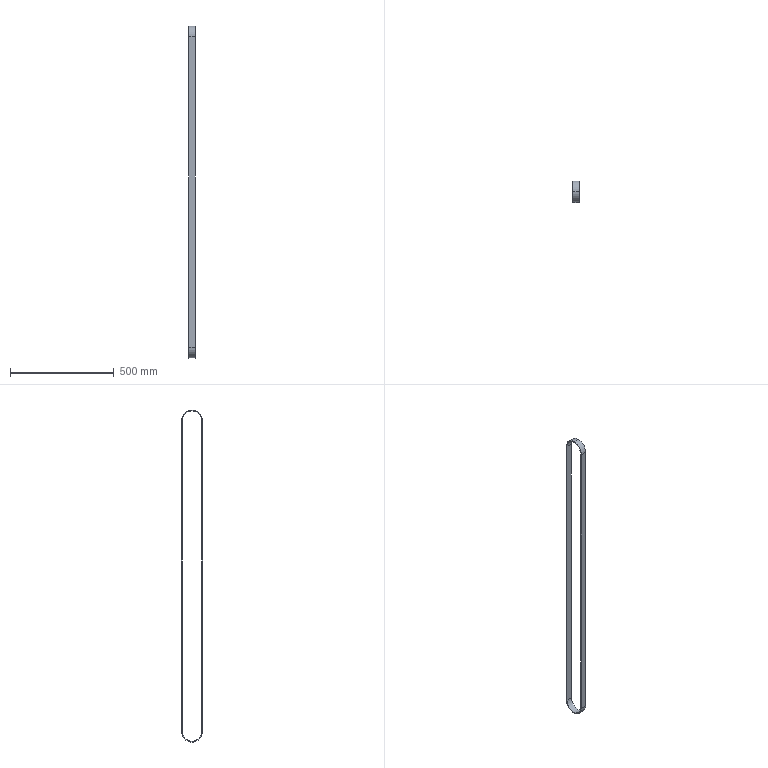Part | SolidWorks | features ExtruThin 1 | 1 solid | 12 faces | box 30 x 102.5 x 1599 mm | volume 445594 mm3 | cylinder 6 | plane 6 | commonest cylinder face diameters 93.5 x3 102.5 x3
STEP:
#1=CARTESIAN_POINT('',(15.,46.75,1496.41));
#2=VERTEX_POINT('',#1);
#3=CARTESIAN_POINT('',(15.,0.,1543.16));
#4=VERTEX_POINT('',#3);
#5=CARTESIAN_POINT('',(15.,0.,1496.41));
#6=DIRECTION('',(1.,0.,0.));
#7=DIRECTION('',(0.,0.,-1.));
#8=AXIS2_PLACEMENT_3D('',#5,#6,#7);
#9=CIRCLE('',#8,46.75);
#10=EDGE_CURVE('',#2,#4,#9,.T.);
#11=ORIENTED_EDGE('',*,*,#10,.T.);
#12=CARTESIAN_POINT('',(-15.,0.,1543.16));
#13=VERTEX_POINT('',#12);
#14=CARTESIAN_POINT('',(15.,0.,1543.16));
#15=DIRECTION('',(-1.,0.,0.));
#16=VECTOR('',#15,1000.);
#17=LINE('',#14,#16);
#18=EDGE_CURVE('',#4,#13,#17,.T.);
#19=ORIENTED_EDGE('',*,*,#18,.T.);
#20=CARTESIAN_POINT('',(-15.,46.75,1496.41));
#21=VERTEX_POINT('',#20);
#22=CARTESIAN_POINT('',(-15.,0.,1496.41));
#23=DIRECTION('',(1.,0.,0.));
#24=DIRECTION('',(0.,0.,-1.));
#25=AXIS2_PLACEMENT_3D('',#22,#23,#24);
#26=CIRCLE('',#25,46.75);
#27=EDGE_CURVE('',#21,#13,#26,.T.);
#28=ORIENTED_EDGE('',*,*,#27,.F.);
#29=CARTESIAN_POINT('',(15.,46.75,1496.41));
#30=DIRECTION('',(-1.,0.,0.));
#31=VECTOR('',#30,1000.);
#32=LINE('',#29,#31);
#33=EDGE_CURVE('',#2,#21,#32,.T.);
#34=ORIENTED_EDGE('',*,*,#33,.F.);
#35=EDGE_LOOP('',(#11,#19,#28,#34));
#36=FACE_OUTER_BOUND('',#35,.T.);
#37=CARTESIAN_POINT('',(15.,0.,1496.41));
#38=DIRECTION('',(-1.,0.,0.));
#39=DIRECTION('',(0.,0.,1.));
#40=AXIS2_PLACEMENT_3D('',#37,#38,#39);
#41=CYLINDRICAL_SURFACE('',#40,46.75);
#42=ADVANCED_FACE('',(#36),#41,.F.);
#43=CARTESIAN_POINT('',(15.,0.,1547.66));
#44=VERTEX_POINT('',#43);
#45=CARTESIAN_POINT('',(15.,-51.25,1496.41));
#46=VERTEX_POINT('',#45);
#47=CARTESIAN_POINT('',(15.,0.,1496.41));
#48=DIRECTION('',(1.,0.,0.));
#49=DIRECTION('',(0.,0.,-1.));
#50=AXIS2_PLACEMENT_3D('',#47,#48,#49);
#51=CIRCLE('',#50,51.25);
#52=EDGE_CURVE('',#44,#46,#51,.T.);
#53=ORIENTED_EDGE('',*,*,#52,.F.);
#54=CARTESIAN_POINT('',(-15.,0.,1547.66));
#55=VERTEX_POINT('',#54);
#56=CARTESIAN_POINT('',(15.,0.,1547.66));
#57=DIRECTION('',(-1.,0.,0.));
#58=VECTOR('',#57,1000.);
#59=LINE('',#56,#58);
#60=EDGE_CURVE('',#44,#55,#59,.T.);
#61=ORIENTED_EDGE('',*,*,#60,.T.);
#62=CARTESIAN_POINT('',(-15.,-51.25,1496.41));
#63=VERTEX_POINT('',#62);
#64=CARTESIAN_POINT('',(-15.,0.,1496.41));
#65=DIRECTION('',(1.,0.,0.));
#66=DIRECTION('',(0.,0.,-1.));
#67=AXIS2_PLACEMENT_3D('',#64,#65,#66);
#68=CIRCLE('',#67,51.25);
#69=EDGE_CURVE('',#55,#63,#68,.T.);
#70=ORIENTED_EDGE('',*,*,#69,.T.);
#71=CARTESIAN_POINT('',(15.,-51.25,1496.41));
#72=DIRECTION('',(-1.,0.,0.));
#73=VECTOR('',#72,1000.);
#74=LINE('',#71,#73);
#75=EDGE_CURVE('',#46,#63,#74,.T.);
#76=ORIENTED_EDGE('',*,*,#75,.F.);
#77=EDGE_LOOP('',(#53,#61,#70,#76));
#78=FACE_OUTER_BOUND('',#77,.T.);
#79=CARTESIAN_POINT('',(15.,0.,1496.41));
#80=DIRECTION('',(-1.,0.,0.));
#81=DIRECTION('',(0.,0.,1.));
#82=AXIS2_PLACEMENT_3D('',#79,#80,#81);
#83=CYLINDRICAL_SURFACE('',#82,51.25);
#84=ADVANCED_FACE('',(#78),#83,.T.);
#85=CARTESIAN_POINT('',(15.,51.25,1496.41));
#86=VERTEX_POINT('',#85);
#87=CARTESIAN_POINT('',(15.,0.,1496.41));
#88=DIRECTION('',(1.,0.,0.));
#89=DIRECTION('',(0.,0.,-1.));
#90=AXIS2_PLACEMENT_3D('',#87,#88,#89);
#91=CIRCLE('',#90,51.25);
#92=EDGE_CURVE('',#86,#44,#91,.T.);
#93=ORIENTED_EDGE('',*,*,#92,.T.);
#94=ORIENTED_EDGE('',*,*,#52,.T.);
#95=CARTESIAN_POINT('',(15.,-51.25,0.));
#96=VERTEX_POINT('',#95);
#97=CARTESIAN_POINT('',(15.,-51.25,1496.41));
#98=DIRECTION('',(0.,0.,-1.));
#99=VECTOR('',#98,1000.);
#100=LINE('',#97,#99);
#101=EDGE_CURVE('',#46,#96,#100,.T.);
#102=ORIENTED_EDGE('',*,*,#101,.T.);
#103=CARTESIAN_POINT('',(15.,51.25,0.));
#104=VERTEX_POINT('',#103);
#105=CARTESIAN_POINT('',(15.,0.,0.));
#106=DIRECTION('',(1.,0.,0.));
#107=DIRECTION('',(0.,0.,-1.));
#108=AXIS2_PLACEMENT_3D('',#105,#106,#107);
#109=CIRCLE('',#108,51.25);
#110=EDGE_CURVE('',#96,#104,#109,.T.);
#111=ORIENTED_EDGE('',*,*,#110,.T.);
#112=CARTESIAN_POINT('',(15.,51.25,0.));
#113=DIRECTION('',(0.,0.,1.));
#114=VECTOR('',#113,1000.);
#115=LINE('',#112,#114);
#116=EDGE_CURVE('',#104,#86,#115,.T.);
#117=ORIENTED_EDGE('',*,*,#116,.T.);
#118=EDGE_LOOP('',(#93,#94,#102,#111,#117));
#119=FACE_OUTER_BOUND('',#118,.T.);
#120=CARTESIAN_POINT('',(15.,-46.75,1496.41));
#121=VERTEX_POINT('',#120);
#122=CARTESIAN_POINT('',(15.,-46.75,0.));
#123=VERTEX_POINT('',#122);
#124=CARTESIAN_POINT('',(15.,-46.75,1496.41));
#125=DIRECTION('',(0.,0.,-1.));
#126=VECTOR('',#125,1000.);
#127=LINE('',#124,#126);
#128=EDGE_CURVE('',#121,#123,#127,.T.);
#129=ORIENTED_EDGE('',*,*,#128,.F.);
#130=CARTESIAN_POINT('',(15.,0.,1496.41));
#131=DIRECTION('',(1.,0.,0.));
#132=DIRECTION('',(0.,0.,-1.));
#133=AXIS2_PLACEMENT_3D('',#130,#131,#132);
#134=CIRCLE('',#133,46.75);
#135=EDGE_CURVE('',#4,#121,#134,.T.);
#136=ORIENTED_EDGE('',*,*,#135,.F.);
#137=ORIENTED_EDGE('',*,*,#10,.F.);
#138=CARTESIAN_POINT('',(15.,46.75,0.));
#139=VERTEX_POINT('',#138);
#140=CARTESIAN_POINT('',(15.,46.75,0.));
#141=DIRECTION('',(0.,0.,1.));
#142=VECTOR('',#141,1000.);
#143=LINE('',#140,#142);
#144=EDGE_CURVE('',#139,#2,#143,.T.);
#145=ORIENTED_EDGE('',*,*,#144,.F.);
#146=CARTESIAN_POINT('',(15.,0.,0.));
#147=DIRECTION('',(1.,0.,0.));
#148=DIRECTION('',(0.,0.,-1.));
#149=AXIS2_PLACEMENT_3D('',#146,#147,#148);
#150=CIRCLE('',#149,46.75);
#151=EDGE_CURVE('',#123,#139,#150,.T.);
#152=ORIENTED_EDGE('',*,*,#151,.F.);
#153=EDGE_LOOP('',(#129,#136,#137,#145,#152));
#154=FACE_BOUND('',#153,.T.);
#155=CARTESIAN_POINT('',(15.,0.,1496.41));
#156=DIRECTION('',(1.,0.,0.));
#157=DIRECTION('',(0.,0.,-1.));
#158=AXIS2_PLACEMENT_3D('',#155,#156,#157);
#159=PLANE('',#158);
#160=ADVANCED_FACE('',(#119,#154),#159,.T.);
#161=CARTESIAN_POINT('',(-15.,51.25,1496.41));
#162=VERTEX_POINT('',#161);
#163=CARTESIAN_POINT('',(-15.,0.,1496.41));
#164=DIRECTION('',(1.,0.,0.));
#165=DIRECTION('',(0.,0.,-1.));
#166=AXIS2_PLACEMENT_3D('',#163,#164,#165);
#167=CIRCLE('',#166,51.25);
#168=EDGE_CURVE('',#162,#55,#167,.T.);
#169=ORIENTED_EDGE('',*,*,#168,.F.);
#170=CARTESIAN_POINT('',(-15.,51.25,0.));
#171=VERTEX_POINT('',#170);
#172=CARTESIAN_POINT('',(-15.,51.25,0.));
#173=DIRECTION('',(0.,0.,1.));
#174=VECTOR('',#173,1000.);
#175=LINE('',#172,#174);
#176=EDGE_CURVE('',#171,#162,#175,.T.);
#177=ORIENTED_EDGE('',*,*,#176,.F.);
#178=CARTESIAN_POINT('',(-15.,-51.25,0.));
#179=VERTEX_POINT('',#178);
#180=CARTESIAN_POINT('',(-15.,0.,0.));
#181=DIRECTION('',(1.,0.,0.));
#182=DIRECTION('',(0.,0.,-1.));
#183=AXIS2_PLACEMENT_3D('',#180,#181,#182);
#184=CIRCLE('',#183,51.25);
#185=EDGE_CURVE('',#179,#171,#184,.T.);
#186=ORIENTED_EDGE('',*,*,#185,.F.);
#187=CARTESIAN_POINT('',(-15.,-51.25,1496.41));
#188=DIRECTION('',(0.,0.,-1.));
#189=VECTOR('',#188,1000.);
#190=LINE('',#187,#189);
#191=EDGE_CURVE('',#63,#179,#190,.T.);
#192=ORIENTED_EDGE('',*,*,#191,.F.);
#193=ORIENTED_EDGE('',*,*,#69,.F.);
#194=EDGE_LOOP('',(#169,#177,#186,#192,#193));
#195=FACE_OUTER_BOUND('',#194,.T.);
#196=ORIENTED_EDGE('',*,*,#27,.T.);
#197=CARTESIAN_POINT('',(-15.,-46.75,1496.41));
#198=VERTEX_POINT('',#197);
#199=CARTESIAN_POINT('',(-15.,0.,1496.41));
#200=DIRECTION('',(1.,0.,0.));
#201=DIRECTION('',(0.,0.,-1.));
#202=AXIS2_PLACEMENT_3D('',#199,#200,#201);
#203=CIRCLE('',#202,46.75);
#204=EDGE_CURVE('',#13,#198,#203,.T.);
#205=ORIENTED_EDGE('',*,*,#204,.T.);
#206=CARTESIAN_POINT('',(-15.,-46.75,0.));
#207=VERTEX_POINT('',#206);
#208=CARTESIAN_POINT('',(-15.,-46.75,1496.41));
#209=DIRECTION('',(0.,0.,-1.));
#210=VECTOR('',#209,1000.);
#211=LINE('',#208,#210);
#212=EDGE_CURVE('',#198,#207,#211,.T.);
#213=ORIENTED_EDGE('',*,*,#212,.T.);
#214=CARTESIAN_POINT('',(-15.,46.75,0.));
#215=VERTEX_POINT('',#214);
#216=CARTESIAN_POINT('',(-15.,0.,0.));
#217=DIRECTION('',(1.,0.,0.));
#218=DIRECTION('',(0.,0.,-1.));
#219=AXIS2_PLACEMENT_3D('',#216,#217,#218);
#220=CIRCLE('',#219,46.75);
#221=EDGE_CURVE('',#207,#215,#220,.T.);
#222=ORIENTED_EDGE('',*,*,#221,.T.);
#223=CARTESIAN_POINT('',(-15.,46.75,0.));
#224=DIRECTION('',(0.,0.,1.));
#225=VECTOR('',#224,1000.);
#226=LINE('',#223,#225);
#227=EDGE_CURVE('',#215,#21,#226,.T.);
#228=ORIENTED_EDGE('',*,*,#227,.T.);
#229=EDGE_LOOP('',(#196,#205,#213,#222,#228));
#230=FACE_BOUND('',#229,.T.);
#231=CARTESIAN_POINT('',(-15.,0.,1496.41));
#232=DIRECTION('',(1.,0.,0.));
#233=DIRECTION('',(0.,0.,-1.));
#234=AXIS2_PLACEMENT_3D('',#231,#232,#233);
#235=PLANE('',#234);
#236=ADVANCED_FACE('',(#195,#230),#235,.F.);
#237=ORIENTED_EDGE('',*,*,#60,.F.);
#238=ORIENTED_EDGE('',*,*,#92,.F.);
#239=CARTESIAN_POINT('',(15.,51.25,1496.41));
#240=DIRECTION('',(-1.,0.,0.));
#241=VECTOR('',#240,1000.);
#242=LINE('',#239,#241);
#243=EDGE_CURVE('',#86,#162,#242,.T.);
#244=ORIENTED_EDGE('',*,*,#243,.T.);
#245=ORIENTED_EDGE('',*,*,#168,.T.);
#246=EDGE_LOOP('',(#237,#238,#244,#245));
#247=FACE_OUTER_BOUND('',#246,.T.);
#248=CARTESIAN_POINT('',(15.,0.,1496.41));
#249=DIRECTION('',(-1.,0.,0.));
#250=DIRECTION('',(0.,0.,1.));
#251=AXIS2_PLACEMENT_3D('',#248,#249,#250);
#252=CYLINDRICAL_SURFACE('',#251,51.25);
#253=ADVANCED_FACE('',(#247),#252,.T.);
#254=ORIENTED_EDGE('',*,*,#191,.T.);
#255=CARTESIAN_POINT('',(15.,-51.25,0.));
#256=DIRECTION('',(-1.,0.,0.));
#257=VECTOR('',#256,1000.);
#258=LINE('',#255,#257);
#259=EDGE_CURVE('',#96,#179,#258,.T.);
#260=ORIENTED_EDGE('',*,*,#259,.F.);
#261=ORIENTED_EDGE('',*,*,#101,.F.);
#262=ORIENTED_EDGE('',*,*,#75,.T.);
#263=EDGE_LOOP('',(#254,#260,#261,#262));
#264=FACE_OUTER_BOUND('',#263,.T.);
#265=CARTESIAN_POINT('',(15.,-51.25,1496.41));
#266=DIRECTION('',(0.,1.,0.));
#267=DIRECTION('',(0.,0.,1.));
#268=AXIS2_PLACEMENT_3D('',#265,#266,#267);
#269=PLANE('',#268);
#270=ADVANCED_FACE('',(#264),#269,.F.);
#271=ORIENTED_EDGE('',*,*,#185,.T.);
#272=CARTESIAN_POINT('',(15.,51.25,0.));
#273=DIRECTION('',(-1.,0.,0.));
#274=VECTOR('',#273,1000.);
#275=LINE('',#272,#274);
#276=EDGE_CURVE('',#104,#171,#275,.T.);
#277=ORIENTED_EDGE('',*,*,#276,.F.);
#278=ORIENTED_EDGE('',*,*,#110,.F.);
#279=ORIENTED_EDGE('',*,*,#259,.T.);
#280=EDGE_LOOP('',(#271,#277,#278,#279));
#281=FACE_OUTER_BOUND('',#280,.T.);
#282=CARTESIAN_POINT('',(15.,0.,0.));
#283=DIRECTION('',(-1.,0.,0.));
#284=DIRECTION('',(0.,0.,1.));
#285=AXIS2_PLACEMENT_3D('',#282,#283,#284);
#286=CYLINDRICAL_SURFACE('',#285,51.25);
#287=ADVANCED_FACE('',(#281),#286,.T.);
#288=ORIENTED_EDGE('',*,*,#176,.T.);
#289=ORIENTED_EDGE('',*,*,#243,.F.);
#290=ORIENTED_EDGE('',*,*,#116,.F.);
#291=ORIENTED_EDGE('',*,*,#276,.T.);
#292=EDGE_LOOP('',(#288,#289,#290,#291));
#293=FACE_OUTER_BOUND('',#292,.T.);
#294=CARTESIAN_POINT('',(15.,51.25,0.));
#295=DIRECTION('',(0.,-1.,0.));
#296=DIRECTION('',(0.,0.,-1.));
#297=AXIS2_PLACEMENT_3D('',#294,#295,#296);
#298=PLANE('',#297);
#299=ADVANCED_FACE('',(#293),#298,.F.);
#300=ORIENTED_EDGE('',*,*,#18,.F.);
#301=ORIENTED_EDGE('',*,*,#135,.T.);
#302=CARTESIAN_POINT('',(15.,-46.75,1496.41));
#303=DIRECTION('',(-1.,0.,0.));
#304=VECTOR('',#303,1000.);
#305=LINE('',#302,#304);
#306=EDGE_CURVE('',#121,#198,#305,.T.);
#307=ORIENTED_EDGE('',*,*,#306,.T.);
#308=ORIENTED_EDGE('',*,*,#204,.F.);
#309=EDGE_LOOP('',(#300,#301,#307,#308));
#310=FACE_OUTER_BOUND('',#309,.T.);
#311=CARTESIAN_POINT('',(15.,0.,1496.41));
#312=DIRECTION('',(-1.,0.,0.));
#313=DIRECTION('',(0.,0.,1.));
#314=AXIS2_PLACEMENT_3D('',#311,#312,#313);
#315=CYLINDRICAL_SURFACE('',#314,46.75);
#316=ADVANCED_FACE('',(#310),#315,.F.);
#317=ORIENTED_EDGE('',*,*,#212,.F.);
#318=ORIENTED_EDGE('',*,*,#306,.F.);
#319=ORIENTED_EDGE('',*,*,#128,.T.);
#320=CARTESIAN_POINT('',(15.,-46.75,0.));
#321=DIRECTION('',(-1.,0.,0.));
#322=VECTOR('',#321,1000.);
#323=LINE('',#320,#322);
#324=EDGE_CURVE('',#123,#207,#323,.T.);
#325=ORIENTED_EDGE('',*,*,#324,.T.);
#326=EDGE_LOOP('',(#317,#318,#319,#325));
#327=FACE_OUTER_BOUND('',#326,.T.);
#328=CARTESIAN_POINT('',(15.,-46.75,1496.41));
#329=DIRECTION('',(0.,1.,0.));
#330=DIRECTION('',(0.,0.,1.));
#331=AXIS2_PLACEMENT_3D('',#328,#329,#330);
#332=PLANE('',#331);
#333=ADVANCED_FACE('',(#327),#332,.T.);
#334=ORIENTED_EDGE('',*,*,#221,.F.);
#335=ORIENTED_EDGE('',*,*,#324,.F.);
#336=ORIENTED_EDGE('',*,*,#151,.T.);
#337=CARTESIAN_POINT('',(15.,46.75,0.));
#338=DIRECTION('',(-1.,0.,0.));
#339=VECTOR('',#338,1000.);
#340=LINE('',#337,#339);
#341=EDGE_CURVE('',#139,#215,#340,.T.);
#342=ORIENTED_EDGE('',*,*,#341,.T.);
#343=EDGE_LOOP('',(#334,#335,#336,#342));
#344=FACE_OUTER_BOUND('',#343,.T.);
#345=CARTESIAN_POINT('',(15.,0.,0.));
#346=DIRECTION('',(-1.,0.,0.));
#347=DIRECTION('',(0.,0.,1.));
#348=AXIS2_PLACEMENT_3D('',#345,#346,#347);
#349=CYLINDRICAL_SURFACE('',#348,46.75);
#350=ADVANCED_FACE('',(#344),#349,.F.);
#351=ORIENTED_EDGE('',*,*,#227,.F.);
#352=ORIENTED_EDGE('',*,*,#341,.F.);
#353=ORIENTED_EDGE('',*,*,#144,.T.);
#354=ORIENTED_EDGE('',*,*,#33,.T.);
#355=EDGE_LOOP('',(#351,#352,#353,#354));
#356=FACE_OUTER_BOUND('',#355,.T.);
#357=CARTESIAN_POINT('',(15.,46.75,0.));
#358=DIRECTION('',(0.,-1.,0.));
#359=DIRECTION('',(0.,0.,-1.));
#360=AXIS2_PLACEMENT_3D('',#357,#358,#359);
#361=PLANE('',#360);
#362=ADVANCED_FACE('',(#356),#361,.T.);
#363=CLOSED_SHELL('',(#42,#84,#160,#236,#253,#270,#287,#299,#316,#333,#350,#362));
#364=MANIFOLD_SOLID_BREP('',#363);
#365=CARTESIAN_POINT('',(0.,0.,0.));
#366=DIRECTION('',(0.,0.,1.));
#367=DIRECTION('',(1.,0.,0.));
#368=AXIS2_PLACEMENT_3D('',#365,#366,#367);
#369=(LENGTH_UNIT()NAMED_UNIT(*)SI_UNIT(.MILLI.,.METRE.));
#370=UNCERTAINTY_MEASURE_WITH_UNIT(LENGTH_MEASURE(0.00001),#369,'','');
#371=(NAMED_UNIT(*)PLANE_ANGLE_UNIT()SI_UNIT($,.RADIAN.));
#372=(NAMED_UNIT(*)SI_UNIT($,.STERADIAN.)SOLID_ANGLE_UNIT());
#373=(GEOMETRIC_REPRESENTATION_CONTEXT(3)GLOBAL_UNCERTAINTY_ASSIGNED_CONTEXT((#370))GLOBAL_UNIT_ASSIGNED_CONTEXT((#369,#371,#372))REPRESENTATION_CONTEXT('',''));
#374=ADVANCED_BREP_SHAPE_REPRESENTATION('',(#364,#368),#373);